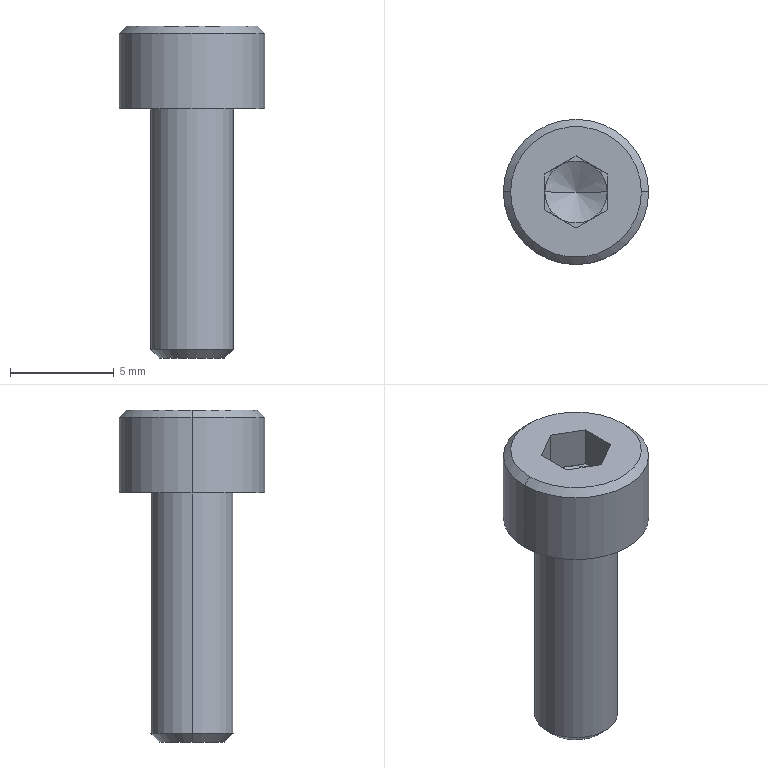Part | STEP file | 1 solid | 25 faces | box 7 x 7 x 16 mm | volume 284.727 mm3 | plane 15 | cone 6 | cylinder 4 | commonest cylinder face diameters 4 x2 7 x2